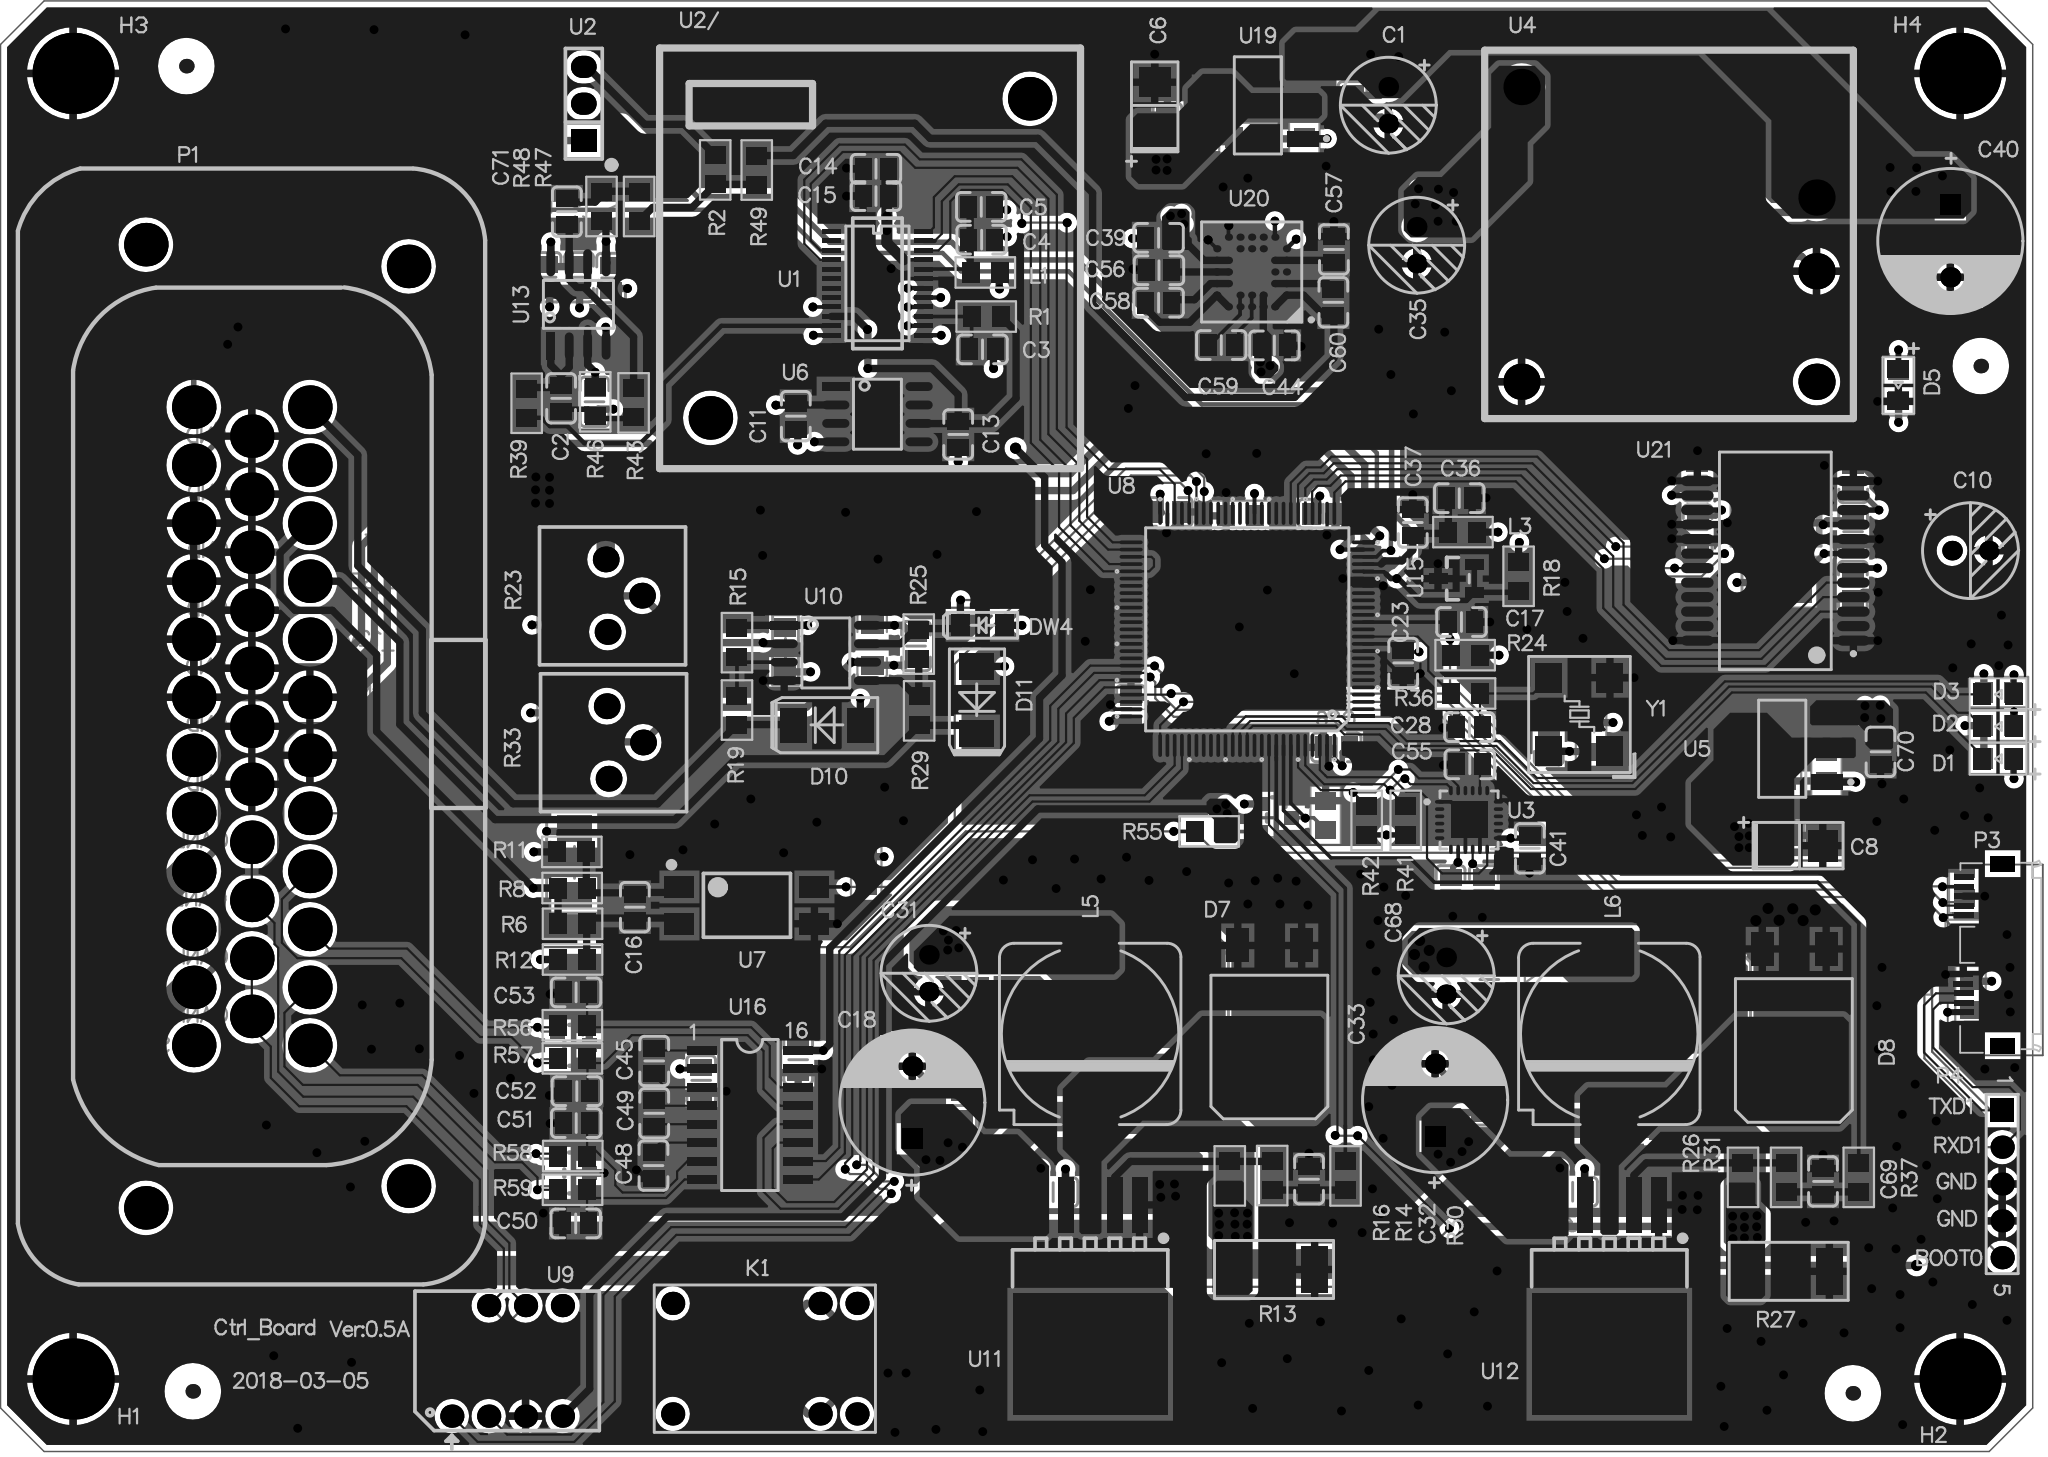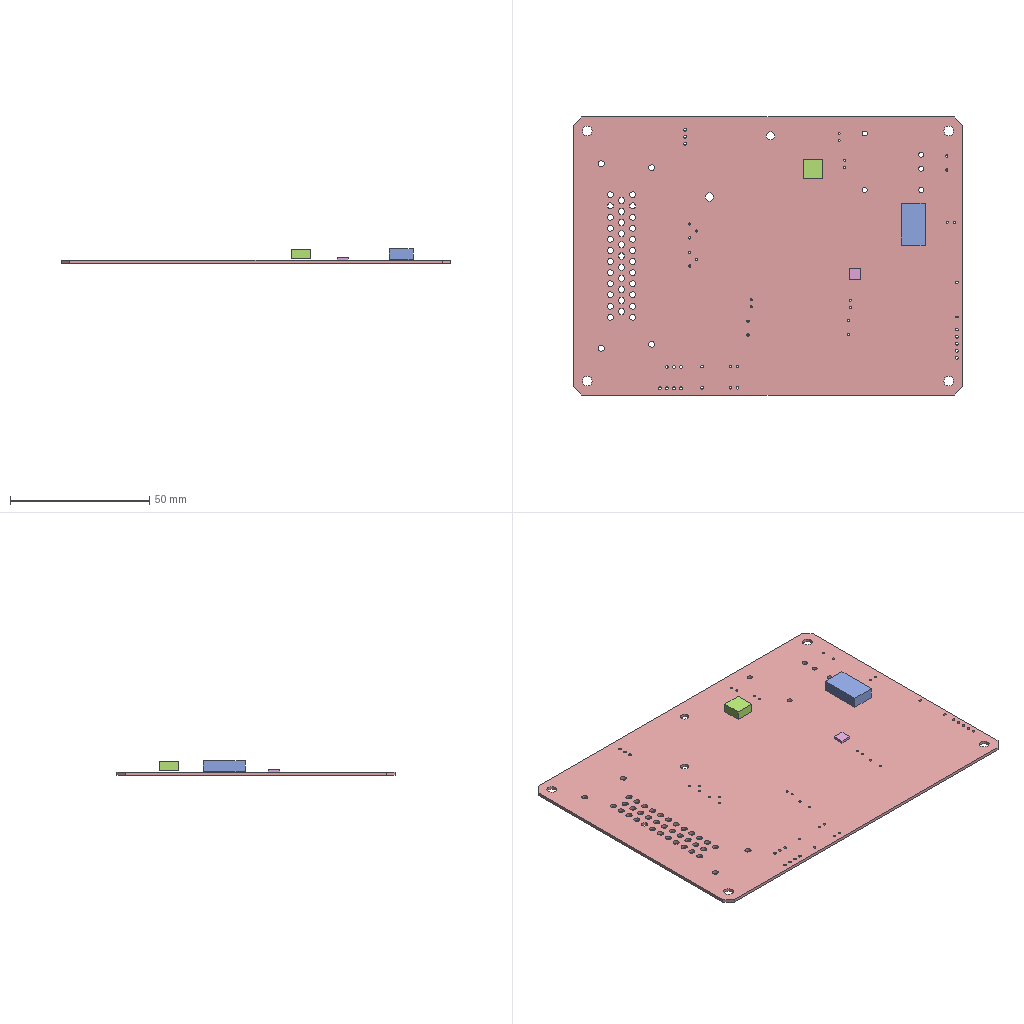Circuit board layout | Altium Designer | box 140 x 100 x 5.3 mm
Layer stack:
# Altium Designer layer stack of  (unit mm; dielectric type: 0 none, 1 core, 2 prepreg, 3 surface material)
index,name,kind,layer,copper_thickness_mm,dielectric_type,dielectric_thickness_mm,dielectric_material,dielectric_constant
0,Top Paste,other,,,,,,
1,Top Overlay,other,,,,,,
2,Top Solder,dielectric,,,3,0.0102,Solder Resist,3.5
3,Top Layer,copper,Top Layer,0.0356,,,,
4,Dielectric1,dielectric,,,1,0.32,FR-4,4.8
5,GND,copper,GND,0.0356,,,,
6,Dielectric5,dielectric,,,2,0.32,FR-4,4.8
7,POWER,copper,POWER,0.0356,,,,
8,Dielectric6,dielectric,,,1,0.32,FR-4,4.8
9,Bottom Layer,copper,Bottom Layer,0.0356,,,,
10,Bottom Solder,dielectric,,,3,0.0102,Solder Resist,3.5
11,Bottom Overlay,other,,,,,,
12,Bottom Paste,other,,,,,,
# drill layer pairs: low layer,high layer
drill_pair,Top Layer,Bottom Layer
Part placement:
Designator,Comment,Layer,Footprint,Center-X(mm),Center-Y(mm),Rotation
R62,0R,BottomLayer,R0805,18.796,94.082,180
R61,10K,BottomLayer,R0805,18.999,80.569,270
R54,0R,BottomLayer,R0805,21.742,80.543,270
C78,100nF,BottomLayer,C0805,16.485,80.772,270
C77,100nF,BottomLayer,C0805,25.908,87.909,270
C76,10uF,BottomLayer,C0805,23.571,87.909,270
U21,SCC2130,TopLayer,SCC2130D,122.27,61.399,180
U20,ADXRS646,TopLayer,ADXRS646,86.192,81.314,180
U19,1117-ADJ,TopLayer,SOT-223,86.621,92.798,90
R35,1K,BottomLayer,R0805,122.997,47.227,90
R27,0.08R,TopLayer,R2512,123.19,12.421,180
R26,1K,TopLayer,R0805,120.04,18.898,90
R21,38.3K,BottomLayer,R0805,89.814,89.611,90
R17,10K,BottomLayer,R0805,86.004,90.551,180
L6,33uH,TopLayer,SLF12555,110.831,28.787,90
L5,33uH,TopLayer,SLF12555,75.067,28.787,90
C70,100nF,TopLayer,C0805,129.515,48.235,90
C69,1uF,TopLayer,C0805,125.552,18.618,90
C68,100uF/25V,TopLayer,RB6.3*7,99.593,32.791,270
C67,470nF,BottomLayer,C0805,127.61,59.665,270
C66,1uF,BottomLayer,C0805,127.635,67.107,90
C65,1uF,BottomLayer,C0805,116.916,63.551,270
C64,100nF,BottomLayer,C0805,127.626,63.409,270
C63,1uF,BottomLayer,C0805,116.891,67.234,90
C62,47uF/10V,BottomLayer,CT3528-B,122.216,64.018,180
C61,47uF/10V,BottomLayer,CT3528-B,122.419,67.981,360
C60,10nF,TopLayer,C0805,91.821,79.223,90
C59,22nF,TopLayer,C0805,84.099,76.276,360
C58,22nF,TopLayer,C0805,79.781,79.197,360
C57,100nF,TopLayer,C0805,91.857,82.864,90
C56,100nF,TopLayer,C0805,79.807,81.432,360
C55,2.2nF,TopLayer,C0805,101.219,47.371,360
C54,100nF,BottomLayer,C0805,102.184,38.684,90
C44,100nF,TopLayer,C0805,87.757,76.251,180
C42,10nF,BottomLayer,C0805,99.898,38.684,90
C41,100nF,TopLayer,C0805,105.359,41.58,90
C40,330µF/35V,TopLayer,CAPPR5.0-10X16-0.8,134.326,83.448,270
C39,100nF,TopLayer,C0805,79.781,83.668,360
C35,100uF/25V,TopLayer,RB6.3*7,97.561,83.16,270
U12,XL3005,TopLayer,TO-263-5,110.831,11.851,90
U11,XL3005,TopLayer,TO-263-5,75.067,11.851,90
U9,CTM1051AM,TopLayer,CTM1051AM,34.9,6.248,360
U3,MPU6050,TopLayer,QFN24,101.168,43.536,360
Y1,8MHZ 3.3V 20PPM,TopLayer,XTAL7050,108.773,50.809,90
U10,LM293DR,TopLayer,SOP-8,56.855,55.05,270
U8,STM32F103VCT6,TopLayer,QFP-100,85.888,56.676,180
U7,PC817,TopLayer,SMD-4,51.42,37.651,360
U6,ADR03A,TopLayer,SOP-8,60.411,71.51,270
U4,E2405UHBDD-10W,TopLayer,E2403UHBDD,114.945,83.905,180
U2,CRS03,TopLayer,HDR1X3,40.183,92.913,90
U1,AD7190BRUZ,TopLayer,IC-24P-TSSOP-6_4MM-G,60.411,80.527,270
R33,100KO potentiometer,TopLayer,CHANGER3,43.013,48.878,270
R23,100KO potentiometer,TopLayer,CHANGER3,42.942,58.998,270
Q2,8550,BottomLayer,SOT-23,87.888,43.688,360
P4,2.54 single-row pin header,TopLayer,HDR1X5,137.897,18.44,270
P1,CON 35-776230-1,TopLayer,VGA35,19.06,49.996,270
D11,P6SMB15A,TopLayer,DO-214,67.269,51.825,270
D10,P6SMB15A,TopLayer,DO-214,56.932,50.072,180
C43,1uF,BottomLayer,C0805,102.565,32.537,270
C38,1uF,BottomLayer,C0805,108.306,17.907,360
C37,10nF,TopLayer,C0805,97.292,64.042,270
C36,1µF,±10%,TopLayer,C0805,100.493,65.719,180
C34,1uF,BottomLayer,C0805,102.083,24.206,90
C33,470µF/25V,TopLayer,CAPPR5.0-10X16-0.8,98.831,24.232,90
C32,1uF,TopLayer,C0805,90.145,18.771,90
C31,100uF/25V,TopLayer,RB6.3*7,63.957,32.969,270
C30,4.7uF/25V,BottomLayer,1206C,60.046,55.601,270
C29,100nF,BottomLayer,C0805,63.068,55.524,270
C28,15pF,TopLayer,C0805,101.194,49.936,360
C27,100nF,BottomLayer,C0805,80.391,64.77,360
C26,100nF,BottomLayer,C0805,92.024,48.539,180
C25,100nF,BottomLayer,C0805,77.876,51.105,90
C24,100nF,BottomLayer,C0805,91.12,64.652,360
C23,100nF,TopLayer,C0805,96.632,54.365,270
C22,100nF,BottomLayer,C0805,106.655,49.022,90
C21,1uF,BottomLayer,C0805,67.31,33.045,270
C20,1uF,BottomLayer,C0805,72.517,17.882,360
C19,1uF,BottomLayer,C0805,66.243,23.851,90
C18,470µF/25V,TopLayer,CAPPR5.0-10X16-0.8,62.814,24.054,90
C17,100nF,TopLayer,C0805,100.645,57.184,180
C15,100nF,TopLayer,C0805,60.31,86.546,180
C14,10uF,TopLayer,C0805,60.31,88.426,180
C13,100nF,TopLayer,C0805,65.974,70.113,270
C12,100nF,BottomLayer,C0805,122.504,42.469,180
C11,100nF,TopLayer,C0805,54.788,71.374,90
C10,100uF/25V,TopLayer,RB6.3*7,135.712,62.103,360
C9,100nF,BottomLayer,C0805,80.391,91.237,270
C7,100nF,BottomLayer,C0805,93.142,92.735,90
C5,100nF,TopLayer,C0805,67.564,85.801,360
C4,10uF,TopLayer,C0805,67.589,83.541,360
C3,10nF,TopLayer,C0805,67.65,75.98,360
C2,22nF,TopLayer,C0805,38.618,72.602,270
C1,100uF/25V,TopLayer,RB6.3*7,95.606,92.812,270
U17,PESD15VL2BT,BottomLayer,SOT-23,39.482,28,0
U18,PESD15VL2BT,BottomLayer,SOT-23,39.472,19.202,0
C45,100nF,TopLayer,C0805,45.034,26.924,90
C46,100nF,BottomLayer,C0805,54.95,27.009,270
C47,100nF,BottomLayer,C0805,48.27,25.587,270
C48,100nF,TopLayer,C0805,44.983,19.71,270
C49,100nF,TopLayer,C0805,45.034,23.317,90
C50,15pF,TopLayer,C0805,39.624,15.723,180
C51,15pF,TopLayer,C0805,39.66,22.64,180
C52,15pF,TopLayer,C0805,39.7,24.841,180
C53,15pF,TopLayer,C0805,39.649,31.648,180
U16,SP3232EEN,TopLayer,SOP16-6.6,51.623,23.199,360
DW3,ZMM3V3,BottomLayer,SMD-D4148,54.077,55.27,90
DW4,ZMM3V3,TopLayer,SMD-D4148,67.65,56.956,180
D4,P6SMB15A,BottomLayer,DO-214,39.522,40.615,270
C16,1µF,±10%,TopLayer,C0805,43.698,37.525,270
L4,47uH,BottomLayer,R1210,122.572,59.904,360
C6,47uF/10V,TopLayer,CT3528-B,79.512,92.795,90
C8,47uF/10V,TopLayer,CT3528-B,123.937,41.766,360
D1,LED0-RED,TopLayer,LED0805,137.609,47.752,180
D2,LED0-GREEN,TopLayer,LED0805,137.609,49.987,180
D3,LED0-BLUE,TopLayer,LED0805,137.609,52.197,180
D5,LED0-RED,TopLayer,LED0805,130.744,73.491,270
D6,SMCJ18A,BottomLayer,SMC,119.38,84.074,90
L1,1uH,TopLayer,R0805,67.843,81.28,180
L2,1uH,BottomLayer,R0805,109.576,49.251,90
L3,10uH,TopLayer,R0805,100.747,63.382,180
P3,USB3.0-B,TopLayer,Micro_USB3.0-B,136.575,34.249,90
R1,0R,TopLayer,R0805,67.904,78.241,360
R2,0R,TopLayer,R0805,49.236,88.35,90
R3,2K,BottomLayer,R0805,130.759,73.457,270
R4,0R,BottomLayer,R0805,40.691,66.04,180
R5,1K,BottomLayer,R0805,137.635,47.752,180
R6,2K,TopLayer,R0805,39.406,36.382,0
R8,2K,TopLayer,R0805,39.38,38.845,0
R9,10K,BottomLayer,R0805,59.639,40.005,270
R10,1K,BottomLayer,R0805,137.635,52.349,180
R11,10K,TopLayer,R0805,39.355,41.334,180
R12,10K,TopLayer,R0805,39.406,33.918,180
R13,0.08R,TopLayer,R2512,87.732,12.548,180
R14,14K,TopLayer,R0805,87.605,19.025,270
R15,100K,TopLayer,R0805,50.734,55.762,270
R16,1K,TopLayer,R0805,84.684,18.999,90
R18,1K,TopLayer,R0805,104.582,60.334,270
R19,10K,TopLayer,R0805,50.734,51.114,270
R20,10K,BottomLayer,R0805,85.43,64.499,360
R22,100K,BottomLayer,R0805,38.039,57.982,270
R24,10K,TopLayer,R0805,100.899,54.898,0
R25,100K,TopLayer,R0805,63.256,55.66,270
R28,10K,BottomLayer,R0805,91.288,43.866,270
R29,10K,TopLayer,R0805,63.285,51.06,270
R30,1K,TopLayer,R0805,92.659,18.999,270
R31,14K,TopLayer,R0805,123.012,18.898,270
R32,100K,BottomLayer,R0805,38.034,49.92,90
R34,10K,BottomLayer,R0805,83.261,42.748,180
R36,10R,TopLayer,R0805,100.924,52.257,0
R37,1K,TopLayer,R0805,128.016,18.898,270
R38,1.6K,BottomLayer,R0805,125.791,47.227,270
R44,10K,BottomLayer,R0805,136.042,35.611,180
R45,10K,BottomLayer,R0805,135.28,39.167,270
R55,10K,TopLayer,R0805,83.261,42.748,360
R56,4.7R,TopLayer,R0805,39.395,29.388,180
R57,4.7R,TopLayer,R0805,39.395,27.102,180
R58,4.7R,TopLayer,R0805,39.421,20.371,180
R59,4.7R,TopLayer,R0805,39.406,18.043,180
R60,0R,BottomLayer,R0805,135.712,31.42,270
U5,1117-ADJ,TopLayer,SOT-223,122.743,48.447,90
D7,MBRD1045,TopLayer,TO-252,87.437,30.813,180
D8,MBRD1045,TopLayer,TO-252,123.571,30.576,180
H1,Hole,TopLayer,HOLE-3.2,5,5,0
H2,Hole,TopLayer,HOLE-3.2,135,5,0
R39,0R,TopLayer,R0805,36.246,72.263,270
R40,120R,BottomLayer,R0805,34.925,7.239,360
R41,10K,TopLayer,R0805,96.808,43.505,270
R42,10K,TopLayer,R0805,94.115,43.505,270
R7,1K,BottomLayer,R0805,137.635,50.038,180
U2/,CRS03,TopLayer,CDS43-01,59.904,82.254,90
C71,22nF,TopLayer,C0805,39.014,85.471,90
C72,22nF,BottomLayer,C0805,40.919,72.365,270
C73,22nF,BottomLayer,C0805,42.062,80.899,270
C74,10uF,BottomLayer,C0805,39.853,80.95,270
C75,100nF,BottomLayer,C0805,37.617,80.95,270
R43,56K 1%,TopLayer,R0805,43.612,72.288,270
R46,91K 1%,TopLayer,R0805,40.97,72.365,90
R47,56K 1%,TopLayer,R0805,43.993,85.827,90
R48,91K 1%,TopLayer,R0805,41.402,85.827,270
R49,0R,TopLayer,R0805,52.095,88.341,90
U13,AD8616ARZ,TopLayer,SOP-8,39.812,79.079,360
D9,MBRD1045,BottomLayer,TO-252,80.594,27.159,180
D12,MBRD1045,BottomLayer,TO-252,116.561,26.701,180
H3,Hole,TopLayer,HOLE-3.2,5,95,0
H4,Hole,TopLayer,HOLE-3.2,135,95,0
D13,1N4148,BottomLayer,SMD-D4148,53.289,6.426,270
K1,HK4100F-DC5V-SHG 0.2W,TopLayer,HK4100F,52.654,6.401,180
R50,1kO,±1%,BottomLayer,0805R,62.484,8.484,270
U14,LMV358IDR,BottomLayer,SOP-8,19.71,87.833,180
Q1,SS8050LT(1.5A),BottomLayer,SOT-23,58.725,6.375,180
U15,TL431AQDBZT,TopLayer,LC-SOT-23(SOT-23-3),100.279,60.173,360
Pad and via stacks:
# Altium Designer via and pad stacks of  (unit mm). Each distinct definition once, with the count of objects using it.
# via: kind,start_layer,end_layer,hole_mm,diameter_mm,mode(0 simple;1 top-mid-bottom;2 full stack),diameter_per_layer,count,example_net
# pad: kind,layer,hole_mm,hole_type(0 round;1 square;2 slot),plating,top_size,top_shape(1 round;2 rect;3 octagon;9 rounded rect),mid_size,bottom_size,mode,footprint,size_per_layer,count,example
pad,Top Layer,0,0,plated,1.524x2.28,2,1.524x2.28,1.524x2.28,0,TO-252,,4,D7.1
pad,Top Layer,0,0,plated,6.74x6.23,2,6.74x6.23,6.74x6.23,0,TO-252,,2,D7.2
pad,Top Layer,0,0,plated,0.4x1.35,2,0.4x1.35,0.4x1.35,0,Micro USB3.0-B,,10,P3.10
pad,Top Layer,0,0,plated,1.2x1.5,2,1.2x1.5,1.2x1.5,0,LED0805,,8,D1.1
pad,Top Layer,0,0,plated,2x2.2,2,2x2.2,2x2.2,0,CT3528-B,,4,C6.1
pad,Top Layer,0,0,plated,1.27x1.5,2,1.27x1.5,1.27x1.5,0,SMD-D4148,,2,DW4.2
pad,Top Layer,0,0,plated,0.6096x2.032,2,0.6096x2.032,0.6096x2.032,0,SOP16-6.6,,16,U16.5
pad,Top Layer,0,0,plated,2.4x1.8,2,2.4x1.8,2.4x1.8,0,DO-214,,4,D11.2
pad,Top Layer,0,0,plated,1.27x0.3048,2,1.27x0.3048,1.27x0.3048,0,IC-24P-TSSOP-6_4MM-G,,24,U1.1
pad,Top Layer,0,0,plated,1.5x2,2,1.5x2,1.5x2,0,SMD-4,,4,U7.4
pad,Top Layer,0,0,plated,1.6x0.254,1,1.6x0.254,1.6x0.254,0,QFP-100,,99,U8.100
pad,Top Layer,0,0,plated,1.6x0.254,2,1.6x0.254,1.6x0.254,0,QFP-100,,1,U8.1
pad,Top Layer,0,0,plated,1.88x0.6096,1,1.88x0.6096,1.88x0.6096,0,SOP-8,,21,U10.8
pad,Top Layer,0,0,plated,1.88x0.6096,2,1.88x0.6096,1.88x0.6096,0,SOP-8,,3,U10.1
pad,Top Layer,0,0,plated,2x1.8,2,2x1.8,2x1.8,0,XTAL7050,,4,Y1.4
pad,Top Layer,0,0,plated,0.25x0.65,1,0.25x0.65,0.25x0.65,0,QFN24,,24,U3.1
pad,Top Layer,0,0,plated,2.5x2.5,2,2.5x2.5,2.5x2.5,0,QFN24,,1,U3.1
pad,Top Layer,0,0,plated,10.65x8.4,2,10.65x8.4,10.65x8.4,0,TO-263-5,,2,U12.0
pad,Top Layer,0,0,plated,1.05x3.8,2,1.05x3.8,1.05x3.8,0,TO-263-5,,10,U12.5
pad,Top Layer,0,0,plated,3x3,2,3x3,3x3,0,SLF12555,,4,L6.2
pad,Top Layer,0,0,plated,1.2x1.4,2,1.2x1.4,1.2x1.4,0,R0805,,68,R26.1
pad,Top Layer,0,0,plated,1.8x3.2,2,1.8x3.2,1.8x3.2,0,R2512,,4,R27.2
pad,Top Layer,0,0,plated,1.1x2.15,2,1.1x2.15,1.1x2.15,0,SOT-223,,6,U19.1
pad,Top Layer,0,0,plated,3.5x2.15,2,3.5x2.15,3.5x2.15,0,SOT-223,,2,U19.2
pad,Top Layer,0,0,plated,0.5x0.5,1,0.5x0.5,0.5x0.5,0,ADXRS646,,32,U20.A2
pad,Top Layer,0,0,plated,0.7x2.25,1,0.7x2.25,0.7x2.25,0,SCC2130D,,24,U21.1
pad,Top Layer,0,0,plated,1x1,1,1x1,1x1,0,,,4,0
pad,Top Layer,0,0,plated,0.7x1.25,2,0.7x1.25,0.7x1.25,0,LC-SOT-23(SOT-23-3),,3,U15.3
pad,Top Layer,0,0,unplated,1.45x1.15,2,1.45x1.15,1.45x1.15,0,C0805,,68,C2.2
pad,Multi-Layer,0.9,0,plated,1.6x1.6,1,1.6x1.6,1.6x1.6,0,HK4100F,,6,K1.1
pad,Multi-Layer,3,0,plated,3x3,1,3x3,3x3,0,CDS43-01,,2,U2/.2
pad,Multi-Layer,3.5,0,plated,5.6x5.6,1,5.6x5.6,5.6x5.6,0,HOLE-3.2,,4,H1.8
pad,Multi-Layer,0.55,2,plated,1.7x1.1,2,1.7x1.1,1.7x1.1,0,Micro USB3.0-B,,2,P3.0
pad,Multi-Layer,2.2,0,plated,3x3,1,3x3,3x3,0,VGA35,,39,P1.1
pad,Multi-Layer,1,0,plated,1.6x1.6,2,1.6x1.6,1.6x1.6,0,HDR1X5,,1,P4.1
pad,Multi-Layer,1,0,plated,1.6x1.6,1,1.6x1.6,1.6x1.6,0,HDR1X5,,4,P4.2
pad,Multi-Layer,0.8,0,plated,1.778x1.778,1,1.778x1.778,1.778x1.778,0,CHANGER3,,6,R33.1
pad,Multi-Layer,1.016,0,plated,1.524x1.778,2,1.524x1.778,1.524x1.778,0,HDR1X3,,1,U2.1
pad,Multi-Layer,1.016,0,plated,1.524x1.778,1,1.524x1.778,1.524x1.778,0,HDR1X3,,2,U2.2
pad,Multi-Layer,1.8,0,plated,2.5x2.5,1,2.5x2.5,2.5x2.5,0,E2403UHBDD,,5,U4.1
pad,Multi-Layer,1,0,plated,1.6x1.6,1,1.6x1.6,1.6x1.6,0,CTM1051AM,,7,U9.1
pad,Multi-Layer,0.8,0,plated,1.4x1.4,2,1.4x1.4,1.4x1.4,0,CAPPR5.0-10X16-0.8,,3,C40.1
pad,Multi-Layer,0.8,0,plated,1.4x1.4,1,1.4x1.4,1.4x1.4,0,CAPPR5.0-10X16-0.8,,3,C40.2
pad,Multi-Layer,0.75,0,plated,1.35x1.35,1,1.35x1.35,1.35x1.35,0,RB6.3*7,,10,C68.2
pad,Bottom Layer,0,0,plated,1.2x1.3,2,1.2x1.3,1.2x1.3,0,0805R,,2,R50.2
pad,Bottom Layer,0,0,plated,2.4x3.3,2,2.4x3.3,2.4x3.3,0,SMC,,2,D6.1
pad,Bottom Layer,0,0,plated,1.6x2.7,2,1.6x2.7,1.6x2.7,0,R1210,,2,L4.1
pad,Bottom Layer,0,0,plated,1.27x1.524,2,1.27x1.524,1.27x1.524,0,1206C,,2,C30.2
pad,Bottom Layer,0,0,plated,0.9144x1.016,2,0.9144x1.016,0.9144x1.016,0,SOT-23,,12,Q2.3
pad,Bottom Layer,0,0,plated,1.2x1.4,2,1.2x1.4,1.2x1.4,0,R0805,,46,R34.1
pad,Bottom Layer,0,0,plated,6.74x6.23,2,6.74x6.23,6.74x6.23,0,TO-252,,2,D9.2
pad,Bottom Layer,0,0,plated,1.524x2.28,2,1.524x2.28,1.524x2.28,0,TO-252,,4,D9.1
pad,Bottom Layer,0,0,plated,2x2.2,2,2x2.2,2x2.2,0,CT3528-B,,4,C62.1
pad,Bottom Layer,0,0,plated,1.27x1.5,2,1.27x1.5,1.27x1.5,0,SMD-D4148,,4,DW3.2
pad,Bottom Layer,0,0,plated,2.4x1.8,2,2.4x1.8,2.4x1.8,0,DO-214,,2,D4.2
pad,Bottom Layer,0,0,plated,1x1,1,1x1,1x1,0,,,4,0
pad,Bottom Layer,0,0,plated,1.88x0.6096,1,1.88x0.6096,1.88x0.6096,0,SOP-8,,7,U14.8
pad,Bottom Layer,0,0,plated,1.88x0.6096,2,1.88x0.6096,1.88x0.6096,0,SOP-8,,1,U14.1
pad,Bottom Layer,0,0,unplated,1.45x1.15,2,1.45x1.15,1.45x1.15,0,C0805,,62,C7.2
via,Top Layer,Bottom Layer,0.3,0.6,0,,144,GND
via,Top Layer,Bottom Layer,0.254,0.508,0,,1,NetD2_1
via,Top Layer,Bottom Layer,0.381,0.762,0,,17,GND
via,Top Layer,Bottom Layer,0.3048,0.6096,0,,278,GND_SB
Copper pours:
name,layer,net,type(0 solid;1 hatched;2 none)
Top Layer-No Net,Top Layer,VDD_5V,0
Top Layer-No Net,Top Layer,VDD_3.3,0
Top Layer-No Net,Top Layer,VDD_5V,0
Top Layer-No Net,Top Layer,VDD_6V,0
Top Layer-No Net,Top Layer,VDD_6V,0
Top Layer-No Net,Top Layer,VDD_6V,0
Top Layer-No Net,Top Layer,SOLENIOD_B,0
Top Layer-No Net,Top Layer,SOLENIOD_A,0
Top Layer-No Net,Top Layer,GND_SA,0
Top Layer-No Net,Top Layer,GND_SB,0
Top Layer-No Net,Top Layer,NetD7_2,0
Top Layer-No Net,Top Layer,NetD8_2,0
Top Layer-No Net,Top Layer,SO_12V,0
Top Layer-No Net,Top Layer,SO_12V,0
Top Layer-No Net,Top Layer,VDD_12V,0
Top Layer-No Net,Top Layer,VDD_3.3,0
Top Layer-No Net,Top Layer,GND,0
Top Layer-No Net,Bottom Layer,GND_SB,0
Top Layer-No Net,Bottom Layer,GND_SA,0
Top Layer-No Net,Bottom Layer,SOLENIOD_A,0
Top Layer-No Net,Bottom Layer,SOLENIOD_B,0
Top Layer-No Net,Bottom Layer,VDD_3.3,0
Top Layer-No Net,Bottom Layer,GND,0
Design rules, without the lines most boards share:
# Altium Designer design rules of  (exported by Altium Designer, unit mm)
# columns: name | kind | enabled | priority | scope1 | scope2 | descriptor | typed fields (field=value)
PolygonConnect_3 | 20 | enabled | 1 | Isvia | All | Polygon Connect Rule(Direct Connect )(Conductor Width=10mil) (Relief Angle=90 Angle) (Entries=4) (Air Gap Width=10mil) (Isvia),(All) | connect_style(0=relief,1=direct,2=none)=1 relief_conductor_width=0.254 relief_entries=4
SilkToSilkClearance | 55 | disabled | 1 | All | All | Silk to Silk (Clearance=10mil) (Disabled)(All),(All) |
SilkscreenOverComponentPads | 54 | disabled | 1 | IsPad | All | Silk To Solder Mask (Clearance=10mil) (Disabled)(IsPad),(All) |
MinimumSolderMaskSliver | 53 | disabled | 1 | All | All | Minimum Solder Mask Sliver (Gap=10mil) (Disabled)(All),(All) |
HoleToHoleClearance | 52 | enabled | 1 | All | All | Hole To Hole Clearance (Gap=10mil) (All),(All) | gap=0.254
DiffPairsRouting | 51 | enabled | 1 | All | All | Differential Pairs Uncoupled Length using the Gap Constraints (Min=10mil) (Max=10mil) (Prefered=10mil)  and Width Constraints (Min=15mil) (Max=15mil) (Prefered=15mil) (All) |
HoleSize | 42 | enabled | 1 | All | All | Hole Size Constraint (Min=1mil) (Max=196.85mil) (All) |
ComponentClearance | 24 | disabled | 1 | All | All | Component Clearance Constraint ( Horizontal Gap = 10mil, Vertical Gap = 10mil ) (Disabled)(All),(All)  | gap=0.254
SolderMaskExpansion | 13 | enabled | 1 | All | All | Solder Mask Expansion (Expansion =4mil) (All) | expansion=0.1016
RoutingVias | 11 | enabled | 1 | All | All | Routing Via (MinHoleWidth=11.811mil) (MaxHoleWidth=28mil) (PreferredHoleWidth=11.811mil) (MinWidth=23.622mil) (MaxWidth=50mil) (PreferedWidth=23.622mil) (All) | via_min_hole=0.3 via_max_hole=0.7112 via_preferred_diameter=0.6 via_preferred_hole=0.3
Width | 2 | enabled | 1 | All | All | Width Constraint (Min=6mil) (Max=80mil) (Preferred=6mil) (All) |
PolygonConnect | 20 | enabled | 4 | All | All | Polygon Connect Rule(Direct Connect )(Conductor Width=7.874mil) (Relief Angle=90 Angle) (Entries=4) (Air Gap Width=10mil) (All),(All) | connect_style(0=relief,1=direct,2=none)=1 relief_conductor_width=0.2 relief_entries=4
PlaneConnect | 6 | enabled | 1 | All | All | Power Plane Connect Rule(Direct Connect )(Expansion=20mil) (Conductor Width=10mil) (Air Gap=10mil) (Entries=4) (All) | relief_conductor_width=0.254 relief_entries=4 relief_expansion=0.508
Clearance | 0 | enabled | 2 | All | All | Clearance Constraint (Gap=6mil) (All),(All) | gap=0.1524
PolygonConnect_1 | 20 | enabled | 3 | InNet('GND') | All | Polygon Connect Rule(Relief Connect )(Conductor Width=20mil) (Relief Angle=90 Angle) (Entries=4) (Air Gap Width=10mil) (InNet('GND')),(All) | connect_style(0=relief,1=direct,2=none)=0 relief_conductor_width=0.508 relief_entries=4
PolygonConnect_2 | 20 | enabled | 2 | InNet('AGND') | All | Polygon Connect Rule(Direct Connect )(Conductor Width=19.685mil) (Relief Angle=90 Angle) (Entries=4) (Air Gap Width=10mil) (InNet('AGND')),(All) | connect_style(0=relief,1=direct,2=none)=1 relief_conductor_width=0.5 relief_entries=4
Clearance_1 | 0 | enabled | 1 | InPolygon | All | Clearance Constraint (Gap=15mil) (InPolygon),(All) | gap=0.381
Classes set for this board:
# Altium Designer classes of  (member kind: 0 net, 1 component, 2 from-to, 3 pad, 4 layer, 5 differential pair, 6 design channel, 7 polygon, 8 structure, 9 xSignal)
# columns: class name | member kind | superclass | members
Ctrl_Board-03-26A | 1 | no | R23; R28; R33; R36; U1; U3; U6; U8; U9; U10; U11; U12; U15; Y1; C28; D10; D11; P1; U2; U4; U5; C1; C2; C3; C4; C5; C6; C7; C8; C9; C10; C11; C12; C13; C14; C15; C17; C18; C19; C20; C21; C22; C23; C24; C25; C26; C27; C28; C29; C30; C31; C32; C33; C34; C36; C37; C38; C43; D1; D2; D3; D4; D5; D6; D7; D8; D10; D11; L1; L2; L3; P1; P3; P4; Q2; R1; R2; R3; R4; R5; R7; R9; R10; R13; R14; R15; R16; R18; R19; R20; R22; R23; R24; R25; R28; R29; R30; R31; R32; R33; R34; R36; R37; R38; R44; R55; U1; U2; U4; U5; U6; U7; U8; U10; U15; Y1; U3; U9; U11; U12; U17; U18; C45; C46; C47; C48; C49; C50; C51; C52; C53; R56; R57; R58; R59; U16; R60; DW3; DW4; H1; H2; R45; U2/; C16; R6; R8; R11; R12; C35; C39; C40; C41; C42; C44; C54; C55; C56; C57; C58; C59; C60; C61; C62; C63; C64; C65; C66; C67; C68; C69; C70; L5; L6; R17; R21; R26; R27; R35; U19; U20; U21; L4; C6; C8; D1; D2; D3; D5; D6; D7; D8; L1; L2; L3; P3; R1; R2; R3; R4; R5; R6; R7; R8; R9; R10; R11; R12; R13; R14; R15; R16; R18; R19; R20; R22; R24; R25; R28; R29; R30; R31; R32; R34; R36; R37; R38; R44; R45; R55; R56; R57; R58; R59; R60; U5; D7; D8; H1; H2; R39; R40; H3; H4; R41; R42; C71; C72; C73; C74; C75; H3; H4; R43; R46; R47; R48; R49; U13; D9; D12; H3; H4; D13; K1; Q3; R50; C76; C77; C78; R54; R61; R62; U14; U15; Q1; U15;